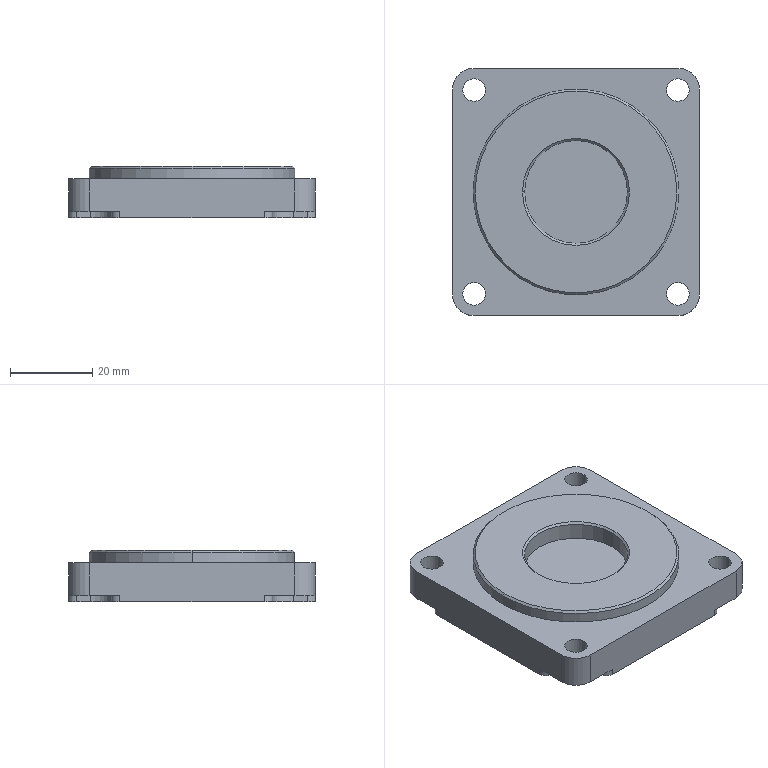Part | STEP file | 31900522--1-SOL000_1_1_1 | 1 solid | 52 faces | box 60 x 60 x 12.5 mm | volume 36244 mm3 | cylinder 28 | plane 20 | cone 4 | commonest cylinder face diameters 4 x8 5.5 x8 10 x8 25 x2 50 x2